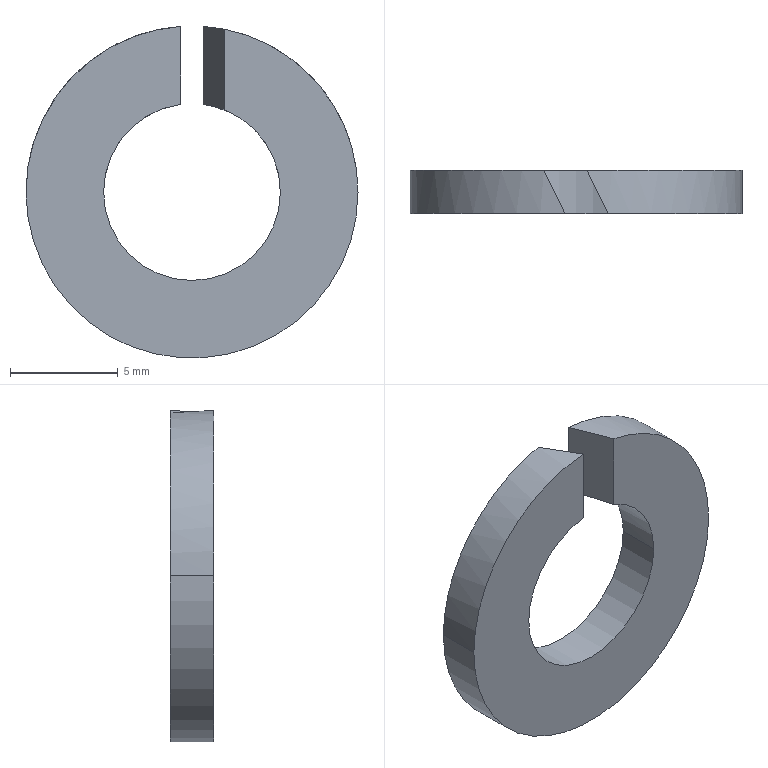Part | STEP file | ZZ24-M8-2 | 1 solid | 10 faces | box 15.4 x 2 x 15.383 mm | volume 252.413 mm3 | cylinder 6 | plane 4 | commonest cylinder face diameters 8.2 x3 15.4 x3
STEP:
#1=CARTESIAN_POINT('',(0.,0.,0.));
#2=DIRECTION('',(0.,0.,1.));
#3=DIRECTION('',(1.,0.,0.));
#4=AXIS2_PLACEMENT_3D('',#1,#2,#3);
#5=CARTESIAN_POINT('',(1.488,0.,3.821));
#6=VERTEX_POINT('',#5);
#7=CARTESIAN_POINT('',(0.5123,2.,4.068));
#8=VERTEX_POINT('',#7);
#9=CARTESIAN_POINT('',(1.488,0.,3.821));
#10=CARTESIAN_POINT('',(1.174,0.6441,3.943));
#11=CARTESIAN_POINT('',(0.8468,1.314,4.026));
#12=CARTESIAN_POINT('',(0.5123,2.,4.068));
#13=(BOUNDED_CURVE()B_SPLINE_CURVE(3,(#9,#10,#11,#12),.UNSPECIFIED.,.F.,.F.)B_SPLINE_CURVE_WITH_KNOTS((4,4),(1.199,1.446),.PIECEWISE_BEZIER_KNOTS.)CURVE()GEOMETRIC_REPRESENTATION_ITEM()RATIONAL_B_SPLINE_CURVE((1.,0.995,0.995,1.))REPRESENTATION_ITEM(''));
#14=CARTESIAN_POINT('',(0.,2.,0.));
#15=DIRECTION('',(0.,-1.,0.));
#16=DIRECTION('',(-1.,0.,0.001512));
#17=AXIS2_PLACEMENT_3D('',#14,#15,#16);
#18=CYLINDRICAL_SURFACE('',#17,4.1);
#19=CARTESIAN_POINT('',(4.343,2.));
#20=CARTESIAN_POINT('',(4.346,1.971));
#21=CARTESIAN_POINT('',(4.354,1.912));
#22=CARTESIAN_POINT('',(4.365,1.824));
#23=CARTESIAN_POINT('',(4.376,1.736));
#24=CARTESIAN_POINT('',(4.387,1.647));
#25=CARTESIAN_POINT('',(4.398,1.558));
#26=CARTESIAN_POINT('',(4.41,1.468));
#27=CARTESIAN_POINT('',(4.421,1.378));
#28=CARTESIAN_POINT('',(4.432,1.288));
#29=CARTESIAN_POINT('',(4.443,1.198));
#30=CARTESIAN_POINT('',(4.454,1.107));
#31=CARTESIAN_POINT('',(4.466,1.016));
#32=CARTESIAN_POINT('',(4.477,0.9243));
#33=CARTESIAN_POINT('',(4.488,0.8327));
#34=CARTESIAN_POINT('',(4.499,0.7408));
#35=CARTESIAN_POINT('',(4.51,0.6487));
#36=CARTESIAN_POINT('',(4.522,0.5565));
#37=CARTESIAN_POINT('',(4.533,0.4641));
#38=CARTESIAN_POINT('',(4.544,0.3715));
#39=CARTESIAN_POINT('',(4.555,0.2788));
#40=CARTESIAN_POINT('',(4.566,0.186));
#41=CARTESIAN_POINT('',(4.577,0.09303));
#42=CARTESIAN_POINT('',(4.585,0.03102));
#43=CARTESIAN_POINT('',(4.589,0.));
#44=B_SPLINE_CURVE_WITH_KNOTS('',3,(#19,#20,#21,#22,#23,#24,#25,#26,#27,#28,#29,#30,#31,#32,#33,#34,#35,#36,#37,#38,#39,#40,#41,#42,#43),.UNSPECIFIED.,.F.,.F.,(4,1,1,1,1,1,1,1,1,1,1,1,1,1,1,1,1,1,1,1,1,1,4),(1.199,1.211,1.222,1.233,1.244,1.255,1.267,1.278,1.289,1.3,1.311,1.322,1.334,1.345,1.356,1.367,1.378,1.39,1.401,1.412,1.423,1.434,1.446),.QUASI_UNIFORM_KNOTS.);
#45=(GEOMETRIC_REPRESENTATION_CONTEXT(2)PARAMETRIC_REPRESENTATION_CONTEXT()REPRESENTATION_CONTEXT('',''));
#46=DEFINITIONAL_REPRESENTATION('',(#44),#45);
#47=PCURVE('',#18,#46);
#48=CARTESIAN_POINT('',(1.488,0.,7.7));
#49=DIRECTION('',(-0.8988,-0.4384,0.));
#50=DIRECTION('',(0.4384,-0.8988,0.));
#51=AXIS2_PLACEMENT_3D('',#48,#49,#50);
#52=PLANE('',#51);
#53=CARTESIAN_POINT('',(0.,-3.879));
#54=CARTESIAN_POINT('',(-0.7167,-3.757));
#55=CARTESIAN_POINT('',(-1.462,-3.674));
#56=CARTESIAN_POINT('',(-2.225,-3.632));
#57=(BOUNDED_CURVE()B_SPLINE_CURVE(3,(#53,#54,#55,#56),.UNSPECIFIED.,.F.,.F.)B_SPLINE_CURVE_WITH_KNOTS((4,4),(1.199,1.446),.PIECEWISE_BEZIER_KNOTS.)CURVE()GEOMETRIC_REPRESENTATION_ITEM()RATIONAL_B_SPLINE_CURVE((1.,0.995,0.995,1.))REPRESENTATION_ITEM(''));
#58=(GEOMETRIC_REPRESENTATION_CONTEXT(2)PARAMETRIC_REPRESENTATION_CONTEXT()REPRESENTATION_CONTEXT('',''));
#59=DEFINITIONAL_REPRESENTATION('',(#57),#58);
#60=PCURVE('',#52,#59);
#61=SURFACE_CURVE('',#13,(#47,#60),.PCURVE_S1.);
#62=EDGE_CURVE('',#6,#8,#61,.T.);
#63=ORIENTED_EDGE('',*,*,#62,.F.);
#64=CARTESIAN_POINT('',(4.1,0.,-0.0062));
#65=VERTEX_POINT('',#64);
#66=CARTESIAN_POINT('',(0.,0.,0.));
#67=DIRECTION('',(0.,1.,0.));
#68=DIRECTION('',(1.,0.,-0.001512));
#69=AXIS2_PLACEMENT_3D('',#66,#67,#68);
#70=CIRCLE('',#69,4.1);
#71=CARTESIAN_POINT('',(9.425,2.));
#72=DIRECTION('',(-1.,0.));
#73=VECTOR('',#72,1.);
#74=LINE('',#71,#73);
#75=(GEOMETRIC_REPRESENTATION_CONTEXT(2)PARAMETRIC_REPRESENTATION_CONTEXT()REPRESENTATION_CONTEXT('',''));
#76=DEFINITIONAL_REPRESENTATION('',(#74),#75);
#77=PCURVE('',#18,#76);
#78=CARTESIAN_POINT('',(0.,0.,0.));
#79=DIRECTION('',(0.,-1.,0.));
#80=DIRECTION('',(-1.,0.,0.001512));
#81=AXIS2_PLACEMENT_3D('',#78,#79,#80);
#82=PLANE('',#81);
#83=CARTESIAN_POINT('',(-4.1,0.));
#84=CARTESIAN_POINT('',(-4.1,7.101));
#85=CARTESIAN_POINT('',(2.05,3.551));
#86=CARTESIAN_POINT('',(8.2,0.));
#87=CARTESIAN_POINT('',(2.05,-3.551));
#88=CARTESIAN_POINT('',(-4.1,-7.101));
#89=CARTESIAN_POINT('',(-4.1,0.));
#90=(BOUNDED_CURVE()B_SPLINE_CURVE(2,(#83,#84,#85,#86,#87,#88,#89),.UNSPECIFIED.,.T.,.F.)B_SPLINE_CURVE_WITH_KNOTS((1,2,2,2,2,1),(-2.094,0.,2.094,4.189,6.283,8.378),.UNSPECIFIED.)CURVE()GEOMETRIC_REPRESENTATION_ITEM()RATIONAL_B_SPLINE_CURVE((1.,0.5,1.,0.5,1.,0.5,1.))REPRESENTATION_ITEM(''));
#91=(GEOMETRIC_REPRESENTATION_CONTEXT(2)PARAMETRIC_REPRESENTATION_CONTEXT()REPRESENTATION_CONTEXT('',''));
#92=DEFINITIONAL_REPRESENTATION('',(#90),#91);
#93=PCURVE('',#82,#92);
#94=SURFACE_CURVE('',#70,(#77,#93),.PCURVE_S1.);
#95=EDGE_CURVE('',#6,#65,#94,.T.);
#96=ORIENTED_EDGE('',*,*,#95,.T.);
#97=CARTESIAN_POINT('',(4.1,2.,-0.0062));
#98=VERTEX_POINT('',#97);
#99=CARTESIAN_POINT('',(4.1,2.,-0.0062));
#100=DIRECTION('',(0.,-1.,0.));
#101=VECTOR('',#100,1.);
#102=LINE('',#99,#101);
#103=CARTESIAN_POINT('',(3.142,0.));
#104=DIRECTION('',(0.,1.));
#105=VECTOR('',#104,1.);
#106=LINE('',#103,#105);
#107=(GEOMETRIC_REPRESENTATION_CONTEXT(2)PARAMETRIC_REPRESENTATION_CONTEXT()REPRESENTATION_CONTEXT('',''));
#108=DEFINITIONAL_REPRESENTATION('',(#106),#107);
#109=PCURVE('',#18,#108);
#110=CARTESIAN_POINT('',(0.,2.,0.));
#111=DIRECTION('',(0.,-1.,0.));
#112=DIRECTION('',(-1.,0.,0.001512));
#113=AXIS2_PLACEMENT_3D('',#110,#111,#112);
#114=CYLINDRICAL_SURFACE('',#113,4.1);
#115=CARTESIAN_POINT('',(3.142,0.));
#116=DIRECTION('',(0.,1.));
#117=VECTOR('',#116,1.);
#118=LINE('',#115,#117);
#119=(GEOMETRIC_REPRESENTATION_CONTEXT(2)PARAMETRIC_REPRESENTATION_CONTEXT()REPRESENTATION_CONTEXT('',''));
#120=DEFINITIONAL_REPRESENTATION('',(#118),#119);
#121=PCURVE('',#114,#120);
#122=SURFACE_CURVE('',#102,(#109,#121),.PCURVE_S1.);
#123=EDGE_CURVE('',#98,#65,#122,.T.);
#124=ORIENTED_EDGE('',*,*,#123,.F.);
#125=CARTESIAN_POINT('',(0.,2.,0.));
#126=DIRECTION('',(0.,-1.,0.));
#127=DIRECTION('',(-1.,0.,0.001512));
#128=AXIS2_PLACEMENT_3D('',#125,#126,#127);
#129=CIRCLE('',#128,4.1);
#130=CARTESIAN_POINT('',(0.,0.));
#131=DIRECTION('',(1.,0.));
#132=VECTOR('',#131,1.);
#133=LINE('',#130,#132);
#134=(GEOMETRIC_REPRESENTATION_CONTEXT(2)PARAMETRIC_REPRESENTATION_CONTEXT()REPRESENTATION_CONTEXT('',''));
#135=DEFINITIONAL_REPRESENTATION('',(#133),#134);
#136=PCURVE('',#18,#135);
#137=CARTESIAN_POINT('',(0.,2.,0.));
#138=DIRECTION('',(0.,1.,0.));
#139=DIRECTION('',(1.,0.,-0.001512));
#140=AXIS2_PLACEMENT_3D('',#137,#138,#139);
#141=PLANE('',#140);
#142=CARTESIAN_POINT('',(-4.1,0.));
#143=CARTESIAN_POINT('',(-4.1,7.101));
#144=CARTESIAN_POINT('',(2.05,3.551));
#145=CARTESIAN_POINT('',(8.2,0.));
#146=CARTESIAN_POINT('',(2.05,-3.551));
#147=CARTESIAN_POINT('',(-4.1,-7.101));
#148=CARTESIAN_POINT('',(-4.1,0.));
#149=(BOUNDED_CURVE()B_SPLINE_CURVE(2,(#142,#143,#144,#145,#146,#147,#148),.UNSPECIFIED.,.T.,.F.)B_SPLINE_CURVE_WITH_KNOTS((1,2,2,2,2,1),(-2.094,0.,2.094,4.189,6.283,8.378),.UNSPECIFIED.)CURVE()GEOMETRIC_REPRESENTATION_ITEM()RATIONAL_B_SPLINE_CURVE((1.,0.5,1.,0.5,1.,0.5,1.))REPRESENTATION_ITEM(''));
#150=(GEOMETRIC_REPRESENTATION_CONTEXT(2)PARAMETRIC_REPRESENTATION_CONTEXT()REPRESENTATION_CONTEXT('',''));
#151=DEFINITIONAL_REPRESENTATION('',(#149),#150);
#152=PCURVE('',#141,#151);
#153=SURFACE_CURVE('',#129,(#136,#152),.PCURVE_S1.);
#154=EDGE_CURVE('',#98,#8,#153,.T.);
#155=ORIENTED_EDGE('',*,*,#154,.T.);
#156=EDGE_LOOP('',(#63,#96,#124,#155));
#157=FACE_BOUND('',#156,.F.);
#158=ADVANCED_FACE('',(#157),#18,.F.);
#159=CARTESIAN_POINT('',(-4.1,0.,0.0062));
#160=VERTEX_POINT('',#159);
#161=CARTESIAN_POINT('',(0.,0.,0.));
#162=DIRECTION('',(0.,1.,0.));
#163=DIRECTION('',(1.,0.,-0.001512));
#164=AXIS2_PLACEMENT_3D('',#161,#162,#163);
#165=CIRCLE('',#164,4.1);
#166=CARTESIAN_POINT('',(3.142,2.));
#167=DIRECTION('',(-1.,0.));
#168=VECTOR('',#167,1.);
#169=LINE('',#166,#168);
#170=(GEOMETRIC_REPRESENTATION_CONTEXT(2)PARAMETRIC_REPRESENTATION_CONTEXT()REPRESENTATION_CONTEXT('',''));
#171=DEFINITIONAL_REPRESENTATION('',(#169),#170);
#172=PCURVE('',#114,#171);
#173=CARTESIAN_POINT('',(-4.1,0.));
#174=CARTESIAN_POINT('',(-4.1,7.101));
#175=CARTESIAN_POINT('',(2.05,3.551));
#176=CARTESIAN_POINT('',(8.2,0.));
#177=CARTESIAN_POINT('',(2.05,-3.551));
#178=CARTESIAN_POINT('',(-4.1,-7.101));
#179=CARTESIAN_POINT('',(-4.1,0.));
#180=(BOUNDED_CURVE()B_SPLINE_CURVE(2,(#173,#174,#175,#176,#177,#178,#179),.UNSPECIFIED.,.T.,.F.)B_SPLINE_CURVE_WITH_KNOTS((1,2,2,2,2,1),(-2.094,0.,2.094,4.189,6.283,8.378),.UNSPECIFIED.)CURVE()GEOMETRIC_REPRESENTATION_ITEM()RATIONAL_B_SPLINE_CURVE((1.,0.5,1.,0.5,1.,0.5,1.))REPRESENTATION_ITEM(''));
#181=(GEOMETRIC_REPRESENTATION_CONTEXT(2)PARAMETRIC_REPRESENTATION_CONTEXT()REPRESENTATION_CONTEXT('',''));
#182=DEFINITIONAL_REPRESENTATION('',(#180),#181);
#183=PCURVE('',#82,#182);
#184=SURFACE_CURVE('',#165,(#172,#183),.PCURVE_S1.);
#185=EDGE_CURVE('',#65,#160,#184,.T.);
#186=ORIENTED_EDGE('',*,*,#185,.T.);
#187=CARTESIAN_POINT('',(-4.1,2.,0.0062));
#188=VERTEX_POINT('',#187);
#189=CARTESIAN_POINT('',(-4.1,2.,0.0062));
#190=DIRECTION('',(0.,-1.,0.));
#191=VECTOR('',#190,1.);
#192=LINE('',#189,#191);
#193=CARTESIAN_POINT('',(0.,0.));
#194=DIRECTION('',(0.,1.));
#195=VECTOR('',#194,1.);
#196=LINE('',#193,#195);
#197=(GEOMETRIC_REPRESENTATION_CONTEXT(2)PARAMETRIC_REPRESENTATION_CONTEXT()REPRESENTATION_CONTEXT('',''));
#198=DEFINITIONAL_REPRESENTATION('',(#196),#197);
#199=PCURVE('',#114,#198);
#200=CARTESIAN_POINT('',(0.,2.,0.));
#201=DIRECTION('',(0.,-1.,0.));
#202=DIRECTION('',(-1.,0.,0.001512));
#203=AXIS2_PLACEMENT_3D('',#200,#201,#202);
#204=CYLINDRICAL_SURFACE('',#203,4.1);
#205=CARTESIAN_POINT('',(6.283,0.));
#206=DIRECTION('',(0.,1.));
#207=VECTOR('',#206,1.);
#208=LINE('',#205,#207);
#209=(GEOMETRIC_REPRESENTATION_CONTEXT(2)PARAMETRIC_REPRESENTATION_CONTEXT()REPRESENTATION_CONTEXT('',''));
#210=DEFINITIONAL_REPRESENTATION('',(#208),#209);
#211=PCURVE('',#204,#210);
#212=SURFACE_CURVE('',#192,(#199,#211),.PCURVE_S1.);
#213=EDGE_CURVE('',#188,#160,#212,.T.);
#214=ORIENTED_EDGE('',*,*,#213,.F.);
#215=CARTESIAN_POINT('',(0.,2.,0.));
#216=DIRECTION('',(0.,-1.,0.));
#217=DIRECTION('',(-1.,0.,0.001512));
#218=AXIS2_PLACEMENT_3D('',#215,#216,#217);
#219=CIRCLE('',#218,4.1);
#220=CARTESIAN_POINT('',(0.,0.));
#221=DIRECTION('',(1.,0.));
#222=VECTOR('',#221,1.);
#223=LINE('',#220,#222);
#224=(GEOMETRIC_REPRESENTATION_CONTEXT(2)PARAMETRIC_REPRESENTATION_CONTEXT()REPRESENTATION_CONTEXT('',''));
#225=DEFINITIONAL_REPRESENTATION('',(#223),#224);
#226=PCURVE('',#114,#225);
#227=CARTESIAN_POINT('',(-4.1,0.));
#228=CARTESIAN_POINT('',(-4.1,7.101));
#229=CARTESIAN_POINT('',(2.05,3.551));
#230=CARTESIAN_POINT('',(8.2,0.));
#231=CARTESIAN_POINT('',(2.05,-3.551));
#232=CARTESIAN_POINT('',(-4.1,-7.101));
#233=CARTESIAN_POINT('',(-4.1,0.));
#234=(BOUNDED_CURVE()B_SPLINE_CURVE(2,(#227,#228,#229,#230,#231,#232,#233),.UNSPECIFIED.,.T.,.F.)B_SPLINE_CURVE_WITH_KNOTS((1,2,2,2,2,1),(-2.094,0.,2.094,4.189,6.283,8.378),.UNSPECIFIED.)CURVE()GEOMETRIC_REPRESENTATION_ITEM()RATIONAL_B_SPLINE_CURVE((1.,0.5,1.,0.5,1.,0.5,1.))REPRESENTATION_ITEM(''));
#235=(GEOMETRIC_REPRESENTATION_CONTEXT(2)PARAMETRIC_REPRESENTATION_CONTEXT()REPRESENTATION_CONTEXT('',''));
#236=DEFINITIONAL_REPRESENTATION('',(#234),#235);
#237=PCURVE('',#141,#236);
#238=SURFACE_CURVE('',#219,(#226,#237),.PCURVE_S1.);
#239=EDGE_CURVE('',#188,#98,#238,.T.);
#240=ORIENTED_EDGE('',*,*,#239,.T.);
#241=ORIENTED_EDGE('',*,*,#123,.T.);
#242=EDGE_LOOP('',(#186,#214,#240,#241));
#243=FACE_BOUND('',#242,.F.);
#244=ADVANCED_FACE('',(#243),#114,.F.);
#245=CARTESIAN_POINT('',(-7.7,2.,0.01164));
#246=VERTEX_POINT('',#245);
#247=CARTESIAN_POINT('',(7.7,2.,-0.01164));
#248=VERTEX_POINT('',#247);
#249=CARTESIAN_POINT('',(0.,2.,0.));
#250=DIRECTION('',(0.,-1.,0.));
#251=DIRECTION('',(-1.,0.,0.001512));
#252=AXIS2_PLACEMENT_3D('',#249,#250,#251);
#253=CIRCLE('',#252,7.7);
#254=CARTESIAN_POINT('',(0.,2.,0.));
#255=DIRECTION('',(0.,-1.,0.));
#256=DIRECTION('',(-1.,0.,0.001512));
#257=AXIS2_PLACEMENT_3D('',#254,#255,#256);
#258=CYLINDRICAL_SURFACE('',#257,7.7);
#259=CARTESIAN_POINT('',(0.,0.));
#260=DIRECTION('',(1.,0.));
#261=VECTOR('',#260,1.);
#262=LINE('',#259,#261);
#263=(GEOMETRIC_REPRESENTATION_CONTEXT(2)PARAMETRIC_REPRESENTATION_CONTEXT()REPRESENTATION_CONTEXT('',''));
#264=DEFINITIONAL_REPRESENTATION('',(#262),#263);
#265=PCURVE('',#258,#264);
#266=CARTESIAN_POINT('',(-7.7,0.));
#267=CARTESIAN_POINT('',(-7.7,13.337));
#268=CARTESIAN_POINT('',(3.85,6.668));
#269=CARTESIAN_POINT('',(15.4,0.));
#270=CARTESIAN_POINT('',(3.85,-6.668));
#271=CARTESIAN_POINT('',(-7.7,-13.337));
#272=CARTESIAN_POINT('',(-7.7,0.));
#273=(BOUNDED_CURVE()B_SPLINE_CURVE(2,(#266,#267,#268,#269,#270,#271,#272),.UNSPECIFIED.,.T.,.F.)B_SPLINE_CURVE_WITH_KNOTS((1,2,2,2,2,1),(-2.094,0.,2.094,4.189,6.283,8.378),.UNSPECIFIED.)CURVE()GEOMETRIC_REPRESENTATION_ITEM()RATIONAL_B_SPLINE_CURVE((1.,0.5,1.,0.5,1.,0.5,1.))REPRESENTATION_ITEM(''));
#274=(GEOMETRIC_REPRESENTATION_CONTEXT(2)PARAMETRIC_REPRESENTATION_CONTEXT()REPRESENTATION_CONTEXT('',''));
#275=DEFINITIONAL_REPRESENTATION('',(#273),#274);
#276=PCURVE('',#141,#275);
#277=SURFACE_CURVE('',#253,(#265,#276),.PCURVE_S1.);
#278=EDGE_CURVE('',#246,#248,#277,.T.);
#279=ORIENTED_EDGE('',*,*,#278,.T.);
#280=CARTESIAN_POINT('',(7.7,0.,-0.01164));
#281=VERTEX_POINT('',#280);
#282=CARTESIAN_POINT('',(7.7,2.,-0.01164));
#283=DIRECTION('',(0.,-1.,0.));
#284=VECTOR('',#283,1.);
#285=LINE('',#282,#284);
#286=CARTESIAN_POINT('',(3.142,0.));
#287=DIRECTION('',(0.,1.));
#288=VECTOR('',#287,1.);
#289=LINE('',#286,#288);
#290=(GEOMETRIC_REPRESENTATION_CONTEXT(2)PARAMETRIC_REPRESENTATION_CONTEXT()REPRESENTATION_CONTEXT('',''));
#291=DEFINITIONAL_REPRESENTATION('',(#289),#290);
#292=PCURVE('',#258,#291);
#293=CARTESIAN_POINT('',(0.,2.,0.));
#294=DIRECTION('',(0.,-1.,0.));
#295=DIRECTION('',(-1.,0.,0.001512));
#296=AXIS2_PLACEMENT_3D('',#293,#294,#295);
#297=CYLINDRICAL_SURFACE('',#296,7.7);
#298=CARTESIAN_POINT('',(3.142,0.));
#299=DIRECTION('',(0.,1.));
#300=VECTOR('',#299,1.);
#301=LINE('',#298,#300);
#302=(GEOMETRIC_REPRESENTATION_CONTEXT(2)PARAMETRIC_REPRESENTATION_CONTEXT()REPRESENTATION_CONTEXT('',''));
#303=DEFINITIONAL_REPRESENTATION('',(#301),#302);
#304=PCURVE('',#297,#303);
#305=SURFACE_CURVE('',#285,(#292,#304),.PCURVE_S1.);
#306=EDGE_CURVE('',#248,#281,#305,.T.);
#307=ORIENTED_EDGE('',*,*,#306,.T.);
#308=CARTESIAN_POINT('',(-7.7,0.,0.01164));
#309=VERTEX_POINT('',#308);
#310=CARTESIAN_POINT('',(0.,0.,0.));
#311=DIRECTION('',(0.,1.,0.));
#312=DIRECTION('',(1.,0.,-0.001512));
#313=AXIS2_PLACEMENT_3D('',#310,#311,#312);
#314=CIRCLE('',#313,7.7);
#315=CARTESIAN_POINT('',(3.142,2.));
#316=DIRECTION('',(-1.,0.));
#317=VECTOR('',#316,1.);
#318=LINE('',#315,#317);
#319=(GEOMETRIC_REPRESENTATION_CONTEXT(2)PARAMETRIC_REPRESENTATION_CONTEXT()REPRESENTATION_CONTEXT('',''));
#320=DEFINITIONAL_REPRESENTATION('',(#318),#319);
#321=PCURVE('',#258,#320);
#322=CARTESIAN_POINT('',(-7.7,0.));
#323=CARTESIAN_POINT('',(-7.7,13.337));
#324=CARTESIAN_POINT('',(3.85,6.668));
#325=CARTESIAN_POINT('',(15.4,0.));
#326=CARTESIAN_POINT('',(3.85,-6.668));
#327=CARTESIAN_POINT('',(-7.7,-13.337));
#328=CARTESIAN_POINT('',(-7.7,0.));
#329=(BOUNDED_CURVE()B_SPLINE_CURVE(2,(#322,#323,#324,#325,#326,#327,#328),.UNSPECIFIED.,.T.,.F.)B_SPLINE_CURVE_WITH_KNOTS((1,2,2,2,2,1),(-2.094,0.,2.094,4.189,6.283,8.378),.UNSPECIFIED.)CURVE()GEOMETRIC_REPRESENTATION_ITEM()RATIONAL_B_SPLINE_CURVE((1.,0.5,1.,0.5,1.,0.5,1.))REPRESENTATION_ITEM(''));
#330=(GEOMETRIC_REPRESENTATION_CONTEXT(2)PARAMETRIC_REPRESENTATION_CONTEXT()REPRESENTATION_CONTEXT('',''));
#331=DEFINITIONAL_REPRESENTATION('',(#329),#330);
#332=PCURVE('',#82,#331);
#333=SURFACE_CURVE('',#314,(#321,#332),.PCURVE_S1.);
#334=EDGE_CURVE('',#281,#309,#333,.T.);
#335=ORIENTED_EDGE('',*,*,#334,.T.);
#336=CARTESIAN_POINT('',(-7.7,2.,0.01164));
#337=DIRECTION('',(0.,-1.,0.));
#338=VECTOR('',#337,1.);
#339=LINE('',#336,#338);
#340=CARTESIAN_POINT('',(0.,0.));
#341=DIRECTION('',(0.,1.));
#342=VECTOR('',#341,1.);
#343=LINE('',#340,#342);
#344=(GEOMETRIC_REPRESENTATION_CONTEXT(2)PARAMETRIC_REPRESENTATION_CONTEXT()REPRESENTATION_CONTEXT('',''));
#345=DEFINITIONAL_REPRESENTATION('',(#343),#344);
#346=PCURVE('',#258,#345);
#347=CARTESIAN_POINT('',(0.,2.,0.));
#348=DIRECTION('',(0.,-1.,0.));
#349=DIRECTION('',(-1.,0.,0.001512));
#350=AXIS2_PLACEMENT_3D('',#347,#348,#349);
#351=CYLINDRICAL_SURFACE('',#350,7.7);
#352=CARTESIAN_POINT('',(6.283,0.));
#353=DIRECTION('',(0.,1.));
#354=VECTOR('',#353,1.);
#355=LINE('',#352,#354);
#356=(GEOMETRIC_REPRESENTATION_CONTEXT(2)PARAMETRIC_REPRESENTATION_CONTEXT()REPRESENTATION_CONTEXT('',''));
#357=DEFINITIONAL_REPRESENTATION('',(#355),#356);
#358=PCURVE('',#351,#357);
#359=SURFACE_CURVE('',#339,(#346,#358),.PCURVE_S1.);
#360=EDGE_CURVE('',#246,#309,#359,.T.);
#361=ORIENTED_EDGE('',*,*,#360,.F.);
#362=EDGE_LOOP('',(#279,#307,#335,#361));
#363=FACE_BOUND('',#362,.T.);
#364=ADVANCED_FACE('',(#363),#258,.T.);
#365=CARTESIAN_POINT('',(-1.488,2.,7.555));
#366=VERTEX_POINT('',#365);
#367=CARTESIAN_POINT('',(0.,2.,0.));
#368=DIRECTION('',(0.,-1.,0.));
#369=DIRECTION('',(-1.,0.,0.001512));
#370=AXIS2_PLACEMENT_3D('',#367,#368,#369);
#371=CIRCLE('',#370,7.7);
#372=CARTESIAN_POINT('',(0.,0.));
#373=DIRECTION('',(1.,0.));
#374=VECTOR('',#373,1.);
#375=LINE('',#372,#374);
#376=(GEOMETRIC_REPRESENTATION_CONTEXT(2)PARAMETRIC_REPRESENTATION_CONTEXT()REPRESENTATION_CONTEXT('',''));
#377=DEFINITIONAL_REPRESENTATION('',(#375),#376);
#378=PCURVE('',#351,#377);
#379=CARTESIAN_POINT('',(-7.7,0.));
#380=CARTESIAN_POINT('',(-7.7,13.337));
#381=CARTESIAN_POINT('',(3.85,6.668));
#382=CARTESIAN_POINT('',(15.4,0.));
#383=CARTESIAN_POINT('',(3.85,-6.668));
#384=CARTESIAN_POINT('',(-7.7,-13.337));
#385=CARTESIAN_POINT('',(-7.7,0.));
#386=(BOUNDED_CURVE()B_SPLINE_CURVE(2,(#379,#380,#381,#382,#383,#384,#385),.UNSPECIFIED.,.T.,.F.)B_SPLINE_CURVE_WITH_KNOTS((1,2,2,2,2,1),(-2.094,0.,2.094,4.189,6.283,8.378),.UNSPECIFIED.)CURVE()GEOMETRIC_REPRESENTATION_ITEM()RATIONAL_B_SPLINE_CURVE((1.,0.5,1.,0.5,1.,0.5,1.))REPRESENTATION_ITEM(''));
#387=(GEOMETRIC_REPRESENTATION_CONTEXT(2)PARAMETRIC_REPRESENTATION_CONTEXT()REPRESENTATION_CONTEXT('',''));
#388=DEFINITIONAL_REPRESENTATION('',(#386),#387);
#389=PCURVE('',#141,#388);
#390=SURFACE_CURVE('',#371,(#378,#389),.PCURVE_S1.);
#391=EDGE_CURVE('',#366,#246,#390,.T.);
#392=ORIENTED_EDGE('',*,*,#391,.T.);
#393=ORIENTED_EDGE('',*,*,#360,.T.);
#394=CARTESIAN_POINT('',(-0.5123,0.,7.683));
#395=VERTEX_POINT('',#394);
#396=CARTESIAN_POINT('',(0.,0.,0.));
#397=DIRECTION('',(0.,1.,0.));
#398=DIRECTION('',(1.,0.,-0.001512));
#399=AXIS2_PLACEMENT_3D('',#396,#397,#398);
#400=CIRCLE('',#399,7.7);
#401=CARTESIAN_POINT('',(9.425,2.));
#402=DIRECTION('',(-1.,0.));
#403=VECTOR('',#402,1.);
#404=LINE('',#401,#403);
#405=(GEOMETRIC_REPRESENTATION_CONTEXT(2)PARAMETRIC_REPRESENTATION_CONTEXT()REPRESENTATION_CONTEXT('',''));
#406=DEFINITIONAL_REPRESENTATION('',(#404),#405);
#407=PCURVE('',#351,#406);
#408=CARTESIAN_POINT('',(-7.7,0.));
#409=CARTESIAN_POINT('',(-7.7,13.337));
#410=CARTESIAN_POINT('',(3.85,6.668));
#411=CARTESIAN_POINT('',(15.4,0.));
#412=CARTESIAN_POINT('',(3.85,-6.668));
#413=CARTESIAN_POINT('',(-7.7,-13.337));
#414=CARTESIAN_POINT('',(-7.7,0.));
#415=(BOUNDED_CURVE()B_SPLINE_CURVE(2,(#408,#409,#410,#411,#412,#413,#414),.UNSPECIFIED.,.T.,.F.)B_SPLINE_CURVE_WITH_KNOTS((1,2,2,2,2,1),(-2.094,0.,2.094,4.189,6.283,8.378),.UNSPECIFIED.)CURVE()GEOMETRIC_REPRESENTATION_ITEM()RATIONAL_B_SPLINE_CURVE((1.,0.5,1.,0.5,1.,0.5,1.))REPRESENTATION_ITEM(''));
#416=(GEOMETRIC_REPRESENTATION_CONTEXT(2)PARAMETRIC_REPRESENTATION_CONTEXT()REPRESENTATION_CONTEXT('',''));
#417=DEFINITIONAL_REPRESENTATION('',(#415),#416);
#418=PCURVE('',#82,#417);
#419=SURFACE_CURVE('',#400,(#407,#418),.PCURVE_S1.);
#420=EDGE_CURVE('',#309,#395,#419,.T.);
#421=ORIENTED_EDGE('',*,*,#420,.T.);
#422=CARTESIAN_POINT('',(-0.5123,0.,7.683));
#423=CARTESIAN_POINT('',(-0.8399,0.6718,7.661));
#424=CARTESIAN_POINT('',(-1.166,1.339,7.618));
#425=CARTESIAN_POINT('',(-1.488,2.,7.555));
#426=(BOUNDED_CURVE()B_SPLINE_CURVE(3,(#422,#423,#424,#425),.UNSPECIFIED.,.F.,.F.)B_SPLINE_CURVE_WITH_KNOTS((4,4),(1.637,1.765),.PIECEWISE_BEZIER_KNOTS.)CURVE()GEOMETRIC_REPRESENTATION_ITEM()RATIONAL_B_SPLINE_CURVE((1.,0.9986,0.9986,1.))REPRESENTATION_ITEM(''));
#427=CARTESIAN_POINT('',(4.78,2.));
#428=CARTESIAN_POINT('',(4.782,1.97));
#429=CARTESIAN_POINT('',(4.786,1.909));
#430=CARTESIAN_POINT('',(4.792,1.817));
#431=CARTESIAN_POINT('',(4.798,1.726));
#432=CARTESIAN_POINT('',(4.804,1.634));
#433=CARTESIAN_POINT('',(4.81,1.543));
#434=CARTESIAN_POINT('',(4.815,1.452));
#435=CARTESIAN_POINT('',(4.821,1.36));
#436=CARTESIAN_POINT('',(4.827,1.269));
#437=CARTESIAN_POINT('',(4.833,1.178));
#438=CARTESIAN_POINT('',(4.839,1.087));
#439=CARTESIAN_POINT('',(4.844,0.9958));
#440=CARTESIAN_POINT('',(4.85,0.9048));
#441=CARTESIAN_POINT('',(4.856,0.8139));
#442=CARTESIAN_POINT('',(4.862,0.7231));
#443=CARTESIAN_POINT('',(4.868,0.6324));
#444=CARTESIAN_POINT('',(4.873,0.5417));
#445=CARTESIAN_POINT('',(4.879,0.4512));
#446=CARTESIAN_POINT('',(4.885,0.3607));
#447=CARTESIAN_POINT('',(4.891,0.2704));
#448=CARTESIAN_POINT('',(4.897,0.1801));
#449=CARTESIAN_POINT('',(4.903,0.09));
#450=CARTESIAN_POINT('',(4.906,0.02999));
#451=CARTESIAN_POINT('',(4.908,0.));
#452=B_SPLINE_CURVE_WITH_KNOTS('',3,(#427,#428,#429,#430,#431,#432,#433,#434,#435,#436,#437,#438,#439,#440,#441,#442,#443,#444,#445,#446,#447,#448,#449,#450,#451),.UNSPECIFIED.,.F.,.F.,(4,1,1,1,1,1,1,1,1,1,1,1,1,1,1,1,1,1,1,1,1,1,4),(1.637,1.643,1.649,1.655,1.661,1.666,1.672,1.678,1.684,1.69,1.695,1.701,1.707,1.713,1.719,1.725,1.73,1.736,1.742,1.748,1.754,1.759,1.765),.QUASI_UNIFORM_KNOTS.);
#453=(GEOMETRIC_REPRESENTATION_CONTEXT(2)PARAMETRIC_REPRESENTATION_CONTEXT()REPRESENTATION_CONTEXT('',''));
#454=DEFINITIONAL_REPRESENTATION('',(#452),#453);
#455=PCURVE('',#351,#454);
#456=CARTESIAN_POINT('',(-1.488,2.,7.7));
#457=DIRECTION('',(0.8988,0.4384,0.));
#458=DIRECTION('',(-0.4384,0.8988,0.));
#459=AXIS2_PLACEMENT_3D('',#456,#457,#458);
#460=PLANE('',#459);
#461=CARTESIAN_POINT('',(-2.225,-0.01706));
#462=CARTESIAN_POINT('',(-1.478,-0.03891));
#463=CARTESIAN_POINT('',(-0.735,-0.08164));
#464=CARTESIAN_POINT('',(0.,-0.1451));
#465=(BOUNDED_CURVE()B_SPLINE_CURVE(3,(#461,#462,#463,#464),.UNSPECIFIED.,.F.,.F.)B_SPLINE_CURVE_WITH_KNOTS((4,4),(1.637,1.765),.PIECEWISE_BEZIER_KNOTS.)CURVE()GEOMETRIC_REPRESENTATION_ITEM()RATIONAL_B_SPLINE_CURVE((1.,0.9986,0.9986,1.))REPRESENTATION_ITEM(''));
#466=(GEOMETRIC_REPRESENTATION_CONTEXT(2)PARAMETRIC_REPRESENTATION_CONTEXT()REPRESENTATION_CONTEXT('',''));
#467=DEFINITIONAL_REPRESENTATION('',(#465),#466);
#468=PCURVE('',#460,#467);
#469=SURFACE_CURVE('',#426,(#455,#468),.PCURVE_S1.);
#470=EDGE_CURVE('',#395,#366,#469,.T.);
#471=ORIENTED_EDGE('',*,*,#470,.T.);
#472=EDGE_LOOP('',(#392,#393,#421,#471));
#473=FACE_BOUND('',#472,.T.);
#474=ADVANCED_FACE('',(#473),#351,.T.);
#475=CARTESIAN_POINT('',(-0.5123,0.,4.068));
#476=VERTEX_POINT('',#475);
#477=CARTESIAN_POINT('',(-0.5123,0.,7.7));
#478=DIRECTION('',(0.,0.,-1.));
#479=VECTOR('',#478,1.);
#480=LINE('',#477,#479);
#481=CARTESIAN_POINT('',(0.5239,-7.699));
#482=DIRECTION('',(-0.001512,1.));
#483=VECTOR('',#482,1.);
#484=LINE('',#481,#483);
#485=(GEOMETRIC_REPRESENTATION_CONTEXT(2)PARAMETRIC_REPRESENTATION_CONTEXT()REPRESENTATION_CONTEXT('',''));
#486=DEFINITIONAL_REPRESENTATION('',(#484),#485);
#487=PCURVE('',#82,#486);
#488=CARTESIAN_POINT('',(-2.225,0.));
#489=DIRECTION('',(0.,-1.));
#490=VECTOR('',#489,1.);
#491=LINE('',#488,#490);
#492=(GEOMETRIC_REPRESENTATION_CONTEXT(2)PARAMETRIC_REPRESENTATION_CONTEXT()REPRESENTATION_CONTEXT('',''));
#493=DEFINITIONAL_REPRESENTATION('',(#491),#492);
#494=PCURVE('',#460,#493);
#495=SURFACE_CURVE('',#480,(#487,#494),.PCURVE_S1.);
#496=EDGE_CURVE('',#395,#476,#495,.T.);
#497=ORIENTED_EDGE('',*,*,#496,.F.);
#498=ORIENTED_EDGE('',*,*,#420,.F.);
#499=ORIENTED_EDGE('',*,*,#334,.F.);
#500=CARTESIAN_POINT('',(1.488,0.,7.555));
#501=VERTEX_POINT('',#500);
#502=CARTESIAN_POINT('',(0.,0.,0.));
#503=DIRECTION('',(0.,1.,0.));
#504=DIRECTION('',(1.,0.,-0.001512));
#505=AXIS2_PLACEMENT_3D('',#502,#503,#504);
#506=CIRCLE('',#505,7.7);
#507=CARTESIAN_POINT('',(-7.7,0.));
#508=CARTESIAN_POINT('',(-7.7,13.337));
#509=CARTESIAN_POINT('',(3.85,6.668));
#510=CARTESIAN_POINT('',(15.4,0.));
#511=CARTESIAN_POINT('',(3.85,-6.668));
#512=CARTESIAN_POINT('',(-7.7,-13.337));
#513=CARTESIAN_POINT('',(-7.7,0.));
#514=(BOUNDED_CURVE()B_SPLINE_CURVE(2,(#507,#508,#509,#510,#511,#512,#513),.UNSPECIFIED.,.T.,.F.)B_SPLINE_CURVE_WITH_KNOTS((1,2,2,2,2,1),(-2.094,0.,2.094,4.189,6.283,8.378),.UNSPECIFIED.)CURVE()GEOMETRIC_REPRESENTATION_ITEM()RATIONAL_B_SPLINE_CURVE((1.,0.5,1.,0.5,1.,0.5,1.))REPRESENTATION_ITEM(''));
#515=(GEOMETRIC_REPRESENTATION_CONTEXT(2)PARAMETRIC_REPRESENTATION_CONTEXT()REPRESENTATION_CONTEXT('',''));
#516=DEFINITIONAL_REPRESENTATION('',(#514),#515);
#517=PCURVE('',#82,#516);
#518=CARTESIAN_POINT('',(9.425,2.));
#519=DIRECTION('',(-1.,0.));
#520=VECTOR('',#519,1.);
#521=LINE('',#518,#520);
#522=(GEOMETRIC_REPRESENTATION_CONTEXT(2)PARAMETRIC_REPRESENTATION_CONTEXT()REPRESENTATION_CONTEXT('',''));
#523=DEFINITIONAL_REPRESENTATION('',(#521),#522);
#524=PCURVE('',#297,#523);
#525=SURFACE_CURVE('',#506,(#517,#524),.PCURVE_S1.);
#526=EDGE_CURVE('',#501,#281,#525,.T.);
#527=ORIENTED_EDGE('',*,*,#526,.F.);
#528=CARTESIAN_POINT('',(1.488,0.,7.7));
#529=DIRECTION('',(0.,0.,-1.));
#530=VECTOR('',#529,1.);
#531=LINE('',#528,#530);
#532=CARTESIAN_POINT('',(-1.476,-7.702));
#533=DIRECTION('',(-0.001512,1.));
#534=VECTOR('',#533,1.);
#535=LINE('',#532,#534);
#536=(GEOMETRIC_REPRESENTATION_CONTEXT(2)PARAMETRIC_REPRESENTATION_CONTEXT()REPRESENTATION_CONTEXT('',''));
#537=DEFINITIONAL_REPRESENTATION('',(#535),#536);
#538=PCURVE('',#82,#537);
#539=CARTESIAN_POINT('',(0.,0.));
#540=DIRECTION('',(0.,-1.));
#541=VECTOR('',#540,1.);
#542=LINE('',#539,#541);
#543=(GEOMETRIC_REPRESENTATION_CONTEXT(2)PARAMETRIC_REPRESENTATION_CONTEXT()REPRESENTATION_CONTEXT('',''));
#544=DEFINITIONAL_REPRESENTATION('',(#542),#543);
#545=PCURVE('',#52,#544);
#546=SURFACE_CURVE('',#531,(#538,#545),.PCURVE_S1.);
#547=EDGE_CURVE('',#501,#6,#546,.T.);
#548=ORIENTED_EDGE('',*,*,#547,.T.);
#549=ORIENTED_EDGE('',*,*,#95,.T.);
#550=ORIENTED_EDGE('',*,*,#185,.T.);
#551=CARTESIAN_POINT('',(0.,0.,0.));
#552=DIRECTION('',(0.,1.,0.));
#553=DIRECTION('',(1.,0.,-0.001512));
#554=AXIS2_PLACEMENT_3D('',#551,#552,#553);
#555=CIRCLE('',#554,4.1);
#556=CARTESIAN_POINT('',(-4.1,0.));
#557=CARTESIAN_POINT('',(-4.1,7.101));
#558=CARTESIAN_POINT('',(2.05,3.551));
#559=CARTESIAN_POINT('',(8.2,0.));
#560=CARTESIAN_POINT('',(2.05,-3.551));
#561=CARTESIAN_POINT('',(-4.1,-7.101));
#562=CARTESIAN_POINT('',(-4.1,0.));
#563=(BOUNDED_CURVE()B_SPLINE_CURVE(2,(#556,#557,#558,#559,#560,#561,#562),.UNSPECIFIED.,.T.,.F.)B_SPLINE_CURVE_WITH_KNOTS((1,2,2,2,2,1),(-2.094,0.,2.094,4.189,6.283,8.378),.UNSPECIFIED.)CURVE()GEOMETRIC_REPRESENTATION_ITEM()RATIONAL_B_SPLINE_CURVE((1.,0.5,1.,0.5,1.,0.5,1.))REPRESENTATION_ITEM(''));
#564=(GEOMETRIC_REPRESENTATION_CONTEXT(2)PARAMETRIC_REPRESENTATION_CONTEXT()REPRESENTATION_CONTEXT('',''));
#565=DEFINITIONAL_REPRESENTATION('',(#563),#564);
#566=PCURVE('',#82,#565);
#567=CARTESIAN_POINT('',(9.425,2.));
#568=DIRECTION('',(-1.,0.));
#569=VECTOR('',#568,1.);
#570=LINE('',#567,#569);
#571=(GEOMETRIC_REPRESENTATION_CONTEXT(2)PARAMETRIC_REPRESENTATION_CONTEXT()REPRESENTATION_CONTEXT('',''));
#572=DEFINITIONAL_REPRESENTATION('',(#570),#571);
#573=PCURVE('',#204,#572);
#574=SURFACE_CURVE('',#555,(#566,#573),.PCURVE_S1.);
#575=EDGE_CURVE('',#160,#476,#574,.T.);
#576=ORIENTED_EDGE('',*,*,#575,.T.);
#577=EDGE_LOOP('',(#497,#498,#499,#527,#548,#549,#550,#576));
#578=FACE_BOUND('',#577,.T.);
#579=ADVANCED_FACE('',(#578),#82,.T.);
#580=CARTESIAN_POINT('',(0.5123,2.,7.683));
#581=VERTEX_POINT('',#580);
#582=CARTESIAN_POINT('',(0.5123,2.,7.7));
#583=DIRECTION('',(0.,0.,-1.));
#584=VECTOR('',#583,1.);
#585=LINE('',#582,#584);
#586=CARTESIAN_POINT('',(0.5006,-7.701));
#587=DIRECTION('',(0.001512,1.));
#588=VECTOR('',#587,1.);
#589=LINE('',#586,#588);
#590=(GEOMETRIC_REPRESENTATION_CONTEXT(2)PARAMETRIC_REPRESENTATION_CONTEXT()REPRESENTATION_CONTEXT('',''));
#591=DEFINITIONAL_REPRESENTATION('',(#589),#590);
#592=PCURVE('',#141,#591);
#593=CARTESIAN_POINT('',(-2.225,0.));
#594=DIRECTION('',(0.,-1.));
#595=VECTOR('',#594,1.);
#596=LINE('',#593,#595);
#597=(GEOMETRIC_REPRESENTATION_CONTEXT(2)PARAMETRIC_REPRESENTATION_CONTEXT()REPRESENTATION_CONTEXT('',''));
#598=DEFINITIONAL_REPRESENTATION('',(#596),#597);
#599=PCURVE('',#52,#598);
#600=SURFACE_CURVE('',#585,(#592,#599),.PCURVE_S1.);
#601=EDGE_CURVE('',#581,#8,#600,.T.);
#602=ORIENTED_EDGE('',*,*,#601,.F.);
#603=CARTESIAN_POINT('',(0.,2.,0.));
#604=DIRECTION('',(0.,-1.,0.));
#605=DIRECTION('',(-1.,0.,0.001512));
#606=AXIS2_PLACEMENT_3D('',#603,#604,#605);
#607=CIRCLE('',#606,7.7);
#608=CARTESIAN_POINT('',(-7.7,0.));
#609=CARTESIAN_POINT('',(-7.7,13.337));
#610=CARTESIAN_POINT('',(3.85,6.668));
#611=CARTESIAN_POINT('',(15.4,0.));
#612=CARTESIAN_POINT('',(3.85,-6.668));
#613=CARTESIAN_POINT('',(-7.7,-13.337));
#614=CARTESIAN_POINT('',(-7.7,0.));
#615=(BOUNDED_CURVE()B_SPLINE_CURVE(2,(#608,#609,#610,#611,#612,#613,#614),.UNSPECIFIED.,.T.,.F.)B_SPLINE_CURVE_WITH_KNOTS((1,2,2,2,2,1),(-2.094,0.,2.094,4.189,6.283,8.378),.UNSPECIFIED.)CURVE()GEOMETRIC_REPRESENTATION_ITEM()RATIONAL_B_SPLINE_CURVE((1.,0.5,1.,0.5,1.,0.5,1.))REPRESENTATION_ITEM(''));
#616=(GEOMETRIC_REPRESENTATION_CONTEXT(2)PARAMETRIC_REPRESENTATION_CONTEXT()REPRESENTATION_CONTEXT('',''));
#617=DEFINITIONAL_REPRESENTATION('',(#615),#616);
#618=PCURVE('',#141,#617);
#619=CARTESIAN_POINT('',(0.,0.));
#620=DIRECTION('',(1.,0.));
#621=VECTOR('',#620,1.);
#622=LINE('',#619,#621);
#623=(GEOMETRIC_REPRESENTATION_CONTEXT(2)PARAMETRIC_REPRESENTATION_CONTEXT()REPRESENTATION_CONTEXT('',''));
#624=DEFINITIONAL_REPRESENTATION('',(#622),#623);
#625=PCURVE('',#297,#624);
#626=SURFACE_CURVE('',#607,(#618,#625),.PCURVE_S1.);
#627=EDGE_CURVE('',#248,#581,#626,.T.);
#628=ORIENTED_EDGE('',*,*,#627,.F.);
#629=ORIENTED_EDGE('',*,*,#278,.F.);
#630=ORIENTED_EDGE('',*,*,#391,.F.);
#631=CARTESIAN_POINT('',(-1.488,2.,3.821));
#632=VERTEX_POINT('',#631);
#633=CARTESIAN_POINT('',(-1.488,2.,7.7));
#634=DIRECTION('',(0.,0.,-1.));
#635=VECTOR('',#634,1.);
#636=LINE('',#633,#635);
#637=CARTESIAN_POINT('',(-1.499,-7.698));
#638=DIRECTION('',(0.001512,1.));
#639=VECTOR('',#638,1.);
#640=LINE('',#637,#639);
#641=(GEOMETRIC_REPRESENTATION_CONTEXT(2)PARAMETRIC_REPRESENTATION_CONTEXT()REPRESENTATION_CONTEXT('',''));
#642=DEFINITIONAL_REPRESENTATION('',(#640),#641);
#643=PCURVE('',#141,#642);
#644=CARTESIAN_POINT('',(0.,0.));
#645=DIRECTION('',(0.,-1.));
#646=VECTOR('',#645,1.);
#647=LINE('',#644,#646);
#648=(GEOMETRIC_REPRESENTATION_CONTEXT(2)PARAMETRIC_REPRESENTATION_CONTEXT()REPRESENTATION_CONTEXT('',''));
#649=DEFINITIONAL_REPRESENTATION('',(#647),#648);
#650=PCURVE('',#460,#649);
#651=SURFACE_CURVE('',#636,(#643,#650),.PCURVE_S1.);
#652=EDGE_CURVE('',#366,#632,#651,.T.);
#653=ORIENTED_EDGE('',*,*,#652,.T.);
#654=CARTESIAN_POINT('',(0.,2.,0.));
#655=DIRECTION('',(0.,-1.,0.));
#656=DIRECTION('',(-1.,0.,0.001512));
#657=AXIS2_PLACEMENT_3D('',#654,#655,#656);
#658=CIRCLE('',#657,4.1);
#659=CARTESIAN_POINT('',(-4.1,0.));
#660=CARTESIAN_POINT('',(-4.1,7.101));
#661=CARTESIAN_POINT('',(2.05,3.551));
#662=CARTESIAN_POINT('',(8.2,0.));
#663=CARTESIAN_POINT('',(2.05,-3.551));
#664=CARTESIAN_POINT('',(-4.1,-7.101));
#665=CARTESIAN_POINT('',(-4.1,0.));
#666=(BOUNDED_CURVE()B_SPLINE_CURVE(2,(#659,#660,#661,#662,#663,#664,#665),.UNSPECIFIED.,.T.,.F.)B_SPLINE_CURVE_WITH_KNOTS((1,2,2,2,2,1),(-2.094,0.,2.094,4.189,6.283,8.378),.UNSPECIFIED.)CURVE()GEOMETRIC_REPRESENTATION_ITEM()RATIONAL_B_SPLINE_CURVE((1.,0.5,1.,0.5,1.,0.5,1.))REPRESENTATION_ITEM(''));
#667=(GEOMETRIC_REPRESENTATION_CONTEXT(2)PARAMETRIC_REPRESENTATION_CONTEXT()REPRESENTATION_CONTEXT('',''));
#668=DEFINITIONAL_REPRESENTATION('',(#666),#667);
#669=PCURVE('',#141,#668);
#670=CARTESIAN_POINT('',(0.,0.));
#671=DIRECTION('',(1.,0.));
#672=VECTOR('',#671,1.);
#673=LINE('',#670,#672);
#674=(GEOMETRIC_REPRESENTATION_CONTEXT(2)PARAMETRIC_REPRESENTATION_CONTEXT()REPRESENTATION_CONTEXT('',''));
#675=DEFINITIONAL_REPRESENTATION('',(#673),#674);
#676=PCURVE('',#204,#675);
#677=SURFACE_CURVE('',#658,(#669,#676),.PCURVE_S1.);
#678=EDGE_CURVE('',#632,#188,#677,.T.);
#679=ORIENTED_EDGE('',*,*,#678,.T.);
#680=ORIENTED_EDGE('',*,*,#239,.T.);
#681=ORIENTED_EDGE('',*,*,#154,.T.);
#682=EDGE_LOOP('',(#602,#628,#629,#630,#653,#679,#680,#681));
#683=FACE_BOUND('',#682,.T.);
#684=ADVANCED_FACE('',(#683),#141,.T.);
#685=ORIENTED_EDGE('',*,*,#306,.F.);
#686=ORIENTED_EDGE('',*,*,#627,.T.);
#687=CARTESIAN_POINT('',(0.5123,2.,7.683));
#688=CARTESIAN_POINT('',(0.8399,1.328,7.661));
#689=CARTESIAN_POINT('',(1.166,0.6606,7.618));
#690=CARTESIAN_POINT('',(1.488,0.,7.555));
#691=(BOUNDED_CURVE()B_SPLINE_CURVE(3,(#687,#688,#689,#690),.UNSPECIFIED.,.F.,.F.)B_SPLINE_CURVE_WITH_KNOTS((4,4),(4.779,4.907),.PIECEWISE_BEZIER_KNOTS.)CURVE()GEOMETRIC_REPRESENTATION_ITEM()RATIONAL_B_SPLINE_CURVE((1.,0.9986,0.9986,1.))REPRESENTATION_ITEM(''));
#692=CARTESIAN_POINT('',(4.647,0.));
#693=CARTESIAN_POINT('',(4.645,0.0305));
#694=CARTESIAN_POINT('',(4.642,0.09148));
#695=CARTESIAN_POINT('',(4.636,0.1829));
#696=CARTESIAN_POINT('',(4.63,0.2744));
#697=CARTESIAN_POINT('',(4.624,0.3658));
#698=CARTESIAN_POINT('',(4.618,0.4571));
#699=CARTESIAN_POINT('',(4.612,0.5484));
#700=CARTESIAN_POINT('',(4.607,0.6397));
#701=CARTESIAN_POINT('',(4.601,0.7309));
#702=CARTESIAN_POINT('',(4.595,0.8221));
#703=CARTESIAN_POINT('',(4.589,0.9132));
#704=CARTESIAN_POINT('',(4.583,1.004));
#705=CARTESIAN_POINT('',(4.578,1.095));
#706=CARTESIAN_POINT('',(4.572,1.186));
#707=CARTESIAN_POINT('',(4.566,1.277));
#708=CARTESIAN_POINT('',(4.56,1.368));
#709=CARTESIAN_POINT('',(4.554,1.458));
#710=CARTESIAN_POINT('',(4.549,1.549));
#711=CARTESIAN_POINT('',(4.543,1.639));
#712=CARTESIAN_POINT('',(4.537,1.73));
#713=CARTESIAN_POINT('',(4.531,1.82));
#714=CARTESIAN_POINT('',(4.525,1.91));
#715=CARTESIAN_POINT('',(4.521,1.97));
#716=CARTESIAN_POINT('',(4.519,2.));
#717=B_SPLINE_CURVE_WITH_KNOTS('',3,(#692,#693,#694,#695,#696,#697,#698,#699,#700,#701,#702,#703,#704,#705,#706,#707,#708,#709,#710,#711,#712,#713,#714,#715,#716),.UNSPECIFIED.,.F.,.F.,(4,1,1,1,1,1,1,1,1,1,1,1,1,1,1,1,1,1,1,1,1,1,4),(4.779,4.785,4.791,4.796,4.802,4.808,4.814,4.82,4.825,4.831,4.837,4.843,4.849,4.855,4.86,4.866,4.872,4.878,4.884,4.889,4.895,4.901,4.907),.QUASI_UNIFORM_KNOTS.);
#718=(GEOMETRIC_REPRESENTATION_CONTEXT(2)PARAMETRIC_REPRESENTATION_CONTEXT()REPRESENTATION_CONTEXT('',''));
#719=DEFINITIONAL_REPRESENTATION('',(#717),#718);
#720=PCURVE('',#297,#719);
#721=CARTESIAN_POINT('',(-2.225,-0.01706));
#722=CARTESIAN_POINT('',(-1.478,-0.03891));
#723=CARTESIAN_POINT('',(-0.735,-0.08164));
#724=CARTESIAN_POINT('',(0.,-0.1451));
#725=(BOUNDED_CURVE()B_SPLINE_CURVE(3,(#721,#722,#723,#724),.UNSPECIFIED.,.F.,.F.)B_SPLINE_CURVE_WITH_KNOTS((4,4),(4.779,4.907),.PIECEWISE_BEZIER_KNOTS.)CURVE()GEOMETRIC_REPRESENTATION_ITEM()RATIONAL_B_SPLINE_CURVE((1.,0.9986,0.9986,1.))REPRESENTATION_ITEM(''));
#726=(GEOMETRIC_REPRESENTATION_CONTEXT(2)PARAMETRIC_REPRESENTATION_CONTEXT()REPRESENTATION_CONTEXT('',''));
#727=DEFINITIONAL_REPRESENTATION('',(#725),#726);
#728=PCURVE('',#52,#727);
#729=SURFACE_CURVE('',#691,(#720,#728),.PCURVE_S1.);
#730=EDGE_CURVE('',#581,#501,#729,.T.);
#731=ORIENTED_EDGE('',*,*,#730,.T.);
#732=ORIENTED_EDGE('',*,*,#526,.T.);
#733=EDGE_LOOP('',(#685,#686,#731,#732));
#734=FACE_BOUND('',#733,.T.);
#735=ADVANCED_FACE('',(#734),#297,.T.);
#736=ORIENTED_EDGE('',*,*,#601,.T.);
#737=ORIENTED_EDGE('',*,*,#62,.F.);
#738=ORIENTED_EDGE('',*,*,#547,.F.);
#739=ORIENTED_EDGE('',*,*,#730,.F.);
#740=EDGE_LOOP('',(#736,#737,#738,#739));
#741=FACE_BOUND('',#740,.T.);
#742=ADVANCED_FACE('',(#741),#52,.T.);
#743=ORIENTED_EDGE('',*,*,#496,.T.);
#744=CARTESIAN_POINT('',(-1.488,2.,3.821));
#745=CARTESIAN_POINT('',(-1.174,1.356,3.943));
#746=CARTESIAN_POINT('',(-0.8468,0.6858,4.026));
#747=CARTESIAN_POINT('',(-0.5123,0.,4.068));
#748=(BOUNDED_CURVE()B_SPLINE_CURVE(3,(#744,#745,#746,#747),.UNSPECIFIED.,.F.,.F.)B_SPLINE_CURVE_WITH_KNOTS((4,4),(4.341,4.587),.PIECEWISE_BEZIER_KNOTS.)CURVE()GEOMETRIC_REPRESENTATION_ITEM()RATIONAL_B_SPLINE_CURVE((1.,0.995,0.995,1.))REPRESENTATION_ITEM(''));
#749=CARTESIAN_POINT('',(0.,-3.879));
#750=CARTESIAN_POINT('',(-0.7167,-3.757));
#751=CARTESIAN_POINT('',(-1.462,-3.674));
#752=CARTESIAN_POINT('',(-2.225,-3.632));
#753=(BOUNDED_CURVE()B_SPLINE_CURVE(3,(#749,#750,#751,#752),.UNSPECIFIED.,.F.,.F.)B_SPLINE_CURVE_WITH_KNOTS((4,4),(4.341,4.587),.PIECEWISE_BEZIER_KNOTS.)CURVE()GEOMETRIC_REPRESENTATION_ITEM()RATIONAL_B_SPLINE_CURVE((1.,0.995,0.995,1.))REPRESENTATION_ITEM(''));
#754=(GEOMETRIC_REPRESENTATION_CONTEXT(2)PARAMETRIC_REPRESENTATION_CONTEXT()REPRESENTATION_CONTEXT('',''));
#755=DEFINITIONAL_REPRESENTATION('',(#753),#754);
#756=PCURVE('',#460,#755);
#757=CARTESIAN_POINT('',(5.085,0.));
#758=CARTESIAN_POINT('',(5.082,0.02913));
#759=CARTESIAN_POINT('',(5.074,0.08754));
#760=CARTESIAN_POINT('',(5.063,0.1756));
#761=CARTESIAN_POINT('',(5.052,0.264));
#762=CARTESIAN_POINT('',(5.041,0.3529));
#763=CARTESIAN_POINT('',(5.029,0.4421));
#764=CARTESIAN_POINT('',(5.018,0.5317));
#765=CARTESIAN_POINT('',(5.007,0.6216));
#766=CARTESIAN_POINT('',(4.996,0.7118));
#767=CARTESIAN_POINT('',(4.985,0.8024));
#768=CARTESIAN_POINT('',(4.973,0.8932));
#769=CARTESIAN_POINT('',(4.962,0.9843));
#770=CARTESIAN_POINT('',(4.951,1.076));
#771=CARTESIAN_POINT('',(4.94,1.167));
#772=CARTESIAN_POINT('',(4.929,1.259));
#773=CARTESIAN_POINT('',(4.917,1.351));
#774=CARTESIAN_POINT('',(4.906,1.444));
#775=CARTESIAN_POINT('',(4.895,1.536));
#776=CARTESIAN_POINT('',(4.884,1.628));
#777=CARTESIAN_POINT('',(4.873,1.721));
#778=CARTESIAN_POINT('',(4.861,1.814));
#779=CARTESIAN_POINT('',(4.85,1.907));
#780=CARTESIAN_POINT('',(4.843,1.969));
#781=CARTESIAN_POINT('',(4.839,2.));
#782=B_SPLINE_CURVE_WITH_KNOTS('',3,(#757,#758,#759,#760,#761,#762,#763,#764,#765,#766,#767,#768,#769,#770,#771,#772,#773,#774,#775,#776,#777,#778,#779,#780,#781),.UNSPECIFIED.,.F.,.F.,(4,1,1,1,1,1,1,1,1,1,1,1,1,1,1,1,1,1,1,1,1,1,4),(4.341,4.352,4.363,4.375,4.386,4.397,4.408,4.419,4.431,4.442,4.453,4.464,4.475,4.486,4.498,4.509,4.52,4.531,4.542,4.554,4.565,4.576,4.587),.QUASI_UNIFORM_KNOTS.);
#783=(GEOMETRIC_REPRESENTATION_CONTEXT(2)PARAMETRIC_REPRESENTATION_CONTEXT()REPRESENTATION_CONTEXT('',''));
#784=DEFINITIONAL_REPRESENTATION('',(#782),#783);
#785=PCURVE('',#204,#784);
#786=SURFACE_CURVE('',#748,(#756,#785),.PCURVE_S1.);
#787=EDGE_CURVE('',#632,#476,#786,.T.);
#788=ORIENTED_EDGE('',*,*,#787,.F.);
#789=ORIENTED_EDGE('',*,*,#652,.F.);
#790=ORIENTED_EDGE('',*,*,#470,.F.);
#791=EDGE_LOOP('',(#743,#788,#789,#790));
#792=FACE_BOUND('',#791,.T.);
#793=ADVANCED_FACE('',(#792),#460,.T.);
#794=ORIENTED_EDGE('',*,*,#575,.T.);
#795=ORIENTED_EDGE('',*,*,#787,.F.);
#796=ORIENTED_EDGE('',*,*,#678,.T.);
#797=ORIENTED_EDGE('',*,*,#213,.T.);
#798=EDGE_LOOP('',(#794,#795,#796,#797));
#799=FACE_BOUND('',#798,.F.);
#800=ADVANCED_FACE('',(#799),#204,.F.);
#801=CLOSED_SHELL('',(#158,#244,#364,#474,#579,#684,#735,#742,#793,#800));
#802=MANIFOLD_SOLID_BREP('',#801);
#803=(LENGTH_UNIT()NAMED_UNIT(*)SI_UNIT(.MILLI.,.METRE.));
#804=UNCERTAINTY_MEASURE_WITH_UNIT(LENGTH_MEASURE(0.0000001),#803,'','');
#805=(NAMED_UNIT(*)PLANE_ANGLE_UNIT()SI_UNIT($,.RADIAN.));
#806=(NAMED_UNIT(*)SI_UNIT($,.STERADIAN.)SOLID_ANGLE_UNIT());
#807=(GEOMETRIC_REPRESENTATION_CONTEXT(3)GLOBAL_UNCERTAINTY_ASSIGNED_CONTEXT((#804))GLOBAL_UNIT_ASSIGNED_CONTEXT((#803,#805,#806))REPRESENTATION_CONTEXT('',''));
#808=ADVANCED_BREP_SHAPE_REPRESENTATION('',(#4,#802),#807);